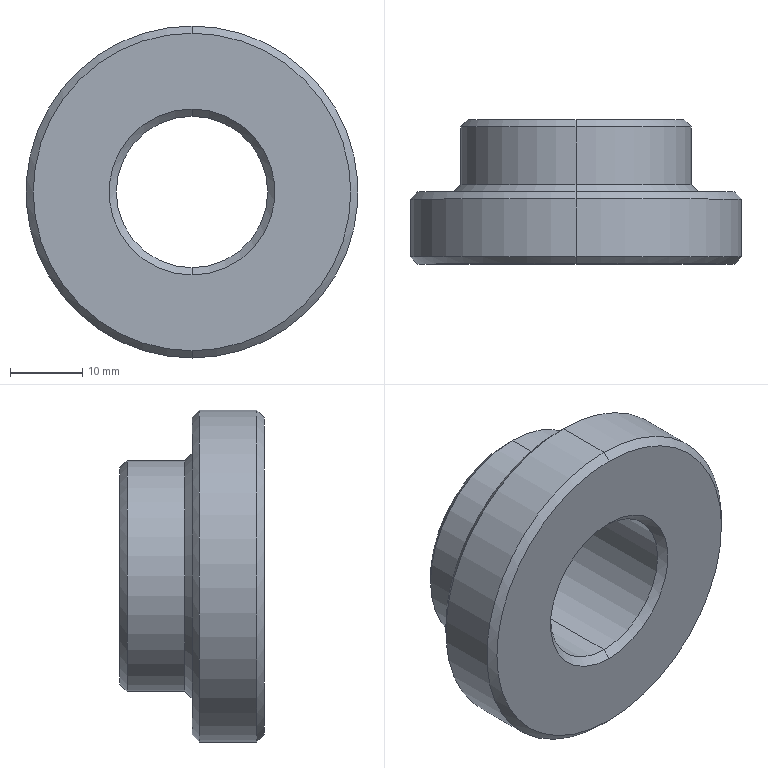Part | SolidWorks | features Chamfer 2, ICE 2, Extrusion 1 | 1 solid | 21 faces | box 46 x 20 x 46 mm | volume 17526 mm3 | cone 12 | cylinder 6 | plane 3 | commonest cylinder face diameters 21 x2 32 x2 46 x2
STEP:
#1=CARTESIAN_POINT('',(0.,1.,10.5));
#2=VERTEX_POINT('',#1);
#3=CARTESIAN_POINT('',(0.,1.,-10.5));
#4=VERTEX_POINT('',#3);
#5=CARTESIAN_POINT('',(0.,1.,0.));
#6=DIRECTION('',(0.,-1.,0.));
#7=DIRECTION('',(0.,0.,1.));
#8=AXIS2_PLACEMENT_3D('',#5,#6,#7);
#9=CIRCLE('',#8,10.5);
#10=EDGE_CURVE('',#2,#4,#9,.T.);
#11=ORIENTED_EDGE('',*,*,#10,.F.);
#12=CARTESIAN_POINT('',(0.,0.,11.5));
#13=VERTEX_POINT('',#12);
#14=CARTESIAN_POINT('',(0.,0.,11.5));
#15=DIRECTION('',(0.,-0.7071,0.7071));
#16=VECTOR('',#15,1000.);
#17=LINE('',#14,#16);
#18=EDGE_CURVE('',#2,#13,#17,.T.);
#19=ORIENTED_EDGE('',*,*,#18,.T.);
#20=CARTESIAN_POINT('',(0.,0.,-11.5));
#21=VERTEX_POINT('',#20);
#22=CARTESIAN_POINT('',(0.,0.,0.));
#23=DIRECTION('',(0.,1.,0.));
#24=DIRECTION('',(0.,0.,1.));
#25=AXIS2_PLACEMENT_3D('',#22,#23,#24);
#26=CIRCLE('',#25,11.5);
#27=EDGE_CURVE('',#21,#13,#26,.T.);
#28=ORIENTED_EDGE('',*,*,#27,.F.);
#29=CARTESIAN_POINT('',(0.,0.,-11.5));
#30=DIRECTION('',(0.,-0.7071,-0.7071));
#31=VECTOR('',#30,1000.);
#32=LINE('',#29,#31);
#33=EDGE_CURVE('',#4,#21,#32,.T.);
#34=ORIENTED_EDGE('',*,*,#33,.F.);
#35=EDGE_LOOP('',(#11,#19,#28,#34));
#36=FACE_OUTER_BOUND('',#35,.T.);
#37=CARTESIAN_POINT('',(0.,0.,0.));
#38=DIRECTION('',(0.,-1.,0.));
#39=DIRECTION('',(0.,0.,-1.));
#40=AXIS2_PLACEMENT_3D('',#37,#38,#39);
#41=CONICAL_SURFACE('',#40,11.5,0.7854);
#42=ADVANCED_FACE('',(#36),#41,.F.);
#43=CARTESIAN_POINT('',(0.,19.,-10.5));
#44=VERTEX_POINT('',#43);
#45=CARTESIAN_POINT('',(0.,19.,10.5));
#46=VERTEX_POINT('',#45);
#47=CARTESIAN_POINT('',(0.,19.,0.));
#48=DIRECTION('',(0.,1.,0.));
#49=DIRECTION('',(0.,0.,1.));
#50=AXIS2_PLACEMENT_3D('',#47,#48,#49);
#51=CIRCLE('',#50,10.5);
#52=EDGE_CURVE('',#44,#46,#51,.T.);
#53=ORIENTED_EDGE('',*,*,#52,.F.);
#54=CARTESIAN_POINT('',(0.,20.,-11.5));
#55=VERTEX_POINT('',#54);
#56=CARTESIAN_POINT('',(0.,19.,-10.5));
#57=DIRECTION('',(0.,0.7071,-0.7071));
#58=VECTOR('',#57,1000.);
#59=LINE('',#56,#58);
#60=EDGE_CURVE('',#44,#55,#59,.T.);
#61=ORIENTED_EDGE('',*,*,#60,.T.);
#62=CARTESIAN_POINT('',(0.,20.,11.5));
#63=VERTEX_POINT('',#62);
#64=CARTESIAN_POINT('',(0.,20.,0.));
#65=DIRECTION('',(0.,-1.,0.));
#66=DIRECTION('',(0.,0.,1.));
#67=AXIS2_PLACEMENT_3D('',#64,#65,#66);
#68=CIRCLE('',#67,11.5);
#69=EDGE_CURVE('',#63,#55,#68,.T.);
#70=ORIENTED_EDGE('',*,*,#69,.F.);
#71=CARTESIAN_POINT('',(0.,19.,10.5));
#72=DIRECTION('',(0.,0.7071,0.7071));
#73=VECTOR('',#72,1000.);
#74=LINE('',#71,#73);
#75=EDGE_CURVE('',#46,#63,#74,.T.);
#76=ORIENTED_EDGE('',*,*,#75,.F.);
#77=EDGE_LOOP('',(#53,#61,#70,#76));
#78=FACE_OUTER_BOUND('',#77,.T.);
#79=CARTESIAN_POINT('',(0.,19.,0.));
#80=DIRECTION('',(0.,1.,0.));
#81=DIRECTION('',(0.,0.,1.));
#82=AXIS2_PLACEMENT_3D('',#79,#80,#81);
#83=CONICAL_SURFACE('',#82,10.5,0.7854);
#84=ADVANCED_FACE('',(#78),#83,.F.);
#85=CARTESIAN_POINT('',(0.,20.,15.));
#86=VERTEX_POINT('',#85);
#87=CARTESIAN_POINT('',(0.,20.,-15.));
#88=VERTEX_POINT('',#87);
#89=CARTESIAN_POINT('',(0.,20.,0.));
#90=DIRECTION('',(0.,1.,0.));
#91=DIRECTION('',(0.,0.,1.));
#92=AXIS2_PLACEMENT_3D('',#89,#90,#91);
#93=CIRCLE('',#92,15.);
#94=EDGE_CURVE('',#86,#88,#93,.T.);
#95=ORIENTED_EDGE('',*,*,#94,.F.);
#96=CARTESIAN_POINT('',(0.,19.,16.));
#97=VERTEX_POINT('',#96);
#98=CARTESIAN_POINT('',(0.,20.,15.));
#99=DIRECTION('',(0.,-0.7071,0.7071));
#100=VECTOR('',#99,1000.);
#101=LINE('',#98,#100);
#102=EDGE_CURVE('',#86,#97,#101,.T.);
#103=ORIENTED_EDGE('',*,*,#102,.T.);
#104=CARTESIAN_POINT('',(0.,19.,-16.));
#105=VERTEX_POINT('',#104);
#106=CARTESIAN_POINT('',(0.,19.,0.));
#107=DIRECTION('',(0.,-1.,0.));
#108=DIRECTION('',(0.,0.,1.));
#109=AXIS2_PLACEMENT_3D('',#106,#107,#108);
#110=CIRCLE('',#109,16.);
#111=EDGE_CURVE('',#105,#97,#110,.T.);
#112=ORIENTED_EDGE('',*,*,#111,.F.);
#113=CARTESIAN_POINT('',(0.,20.,-15.));
#114=DIRECTION('',(0.,-0.7071,-0.7071));
#115=VECTOR('',#114,1000.);
#116=LINE('',#113,#115);
#117=EDGE_CURVE('',#88,#105,#116,.T.);
#118=ORIENTED_EDGE('',*,*,#117,.F.);
#119=EDGE_LOOP('',(#95,#103,#112,#118));
#120=FACE_OUTER_BOUND('',#119,.T.);
#121=CARTESIAN_POINT('',(0.,20.,0.));
#122=DIRECTION('',(0.,-1.,0.));
#123=DIRECTION('',(0.,0.,-1.));
#124=AXIS2_PLACEMENT_3D('',#121,#122,#123);
#125=CONICAL_SURFACE('',#124,15.,0.7854);
#126=ADVANCED_FACE('',(#120),#125,.T.);
#127=CARTESIAN_POINT('',(0.,11.,16.));
#128=VERTEX_POINT('',#127);
#129=CARTESIAN_POINT('',(0.,11.,-16.));
#130=VERTEX_POINT('',#129);
#131=CARTESIAN_POINT('',(0.,11.,0.));
#132=DIRECTION('',(0.,1.,0.));
#133=DIRECTION('',(0.,0.,1.));
#134=AXIS2_PLACEMENT_3D('',#131,#132,#133);
#135=CIRCLE('',#134,16.);
#136=EDGE_CURVE('',#128,#130,#135,.T.);
#137=ORIENTED_EDGE('',*,*,#136,.F.);
#138=CARTESIAN_POINT('',(0.,10.,17.));
#139=VERTEX_POINT('',#138);
#140=CARTESIAN_POINT('',(0.,11.,16.));
#141=DIRECTION('',(0.,-0.7071,0.7071));
#142=VECTOR('',#141,1000.);
#143=LINE('',#140,#142);
#144=EDGE_CURVE('',#128,#139,#143,.T.);
#145=ORIENTED_EDGE('',*,*,#144,.T.);
#146=CARTESIAN_POINT('',(0.,10.,-17.));
#147=VERTEX_POINT('',#146);
#148=CARTESIAN_POINT('',(0.,10.,0.));
#149=DIRECTION('',(0.,-1.,0.));
#150=DIRECTION('',(0.,0.,1.));
#151=AXIS2_PLACEMENT_3D('',#148,#149,#150);
#152=CIRCLE('',#151,17.);
#153=EDGE_CURVE('',#147,#139,#152,.T.);
#154=ORIENTED_EDGE('',*,*,#153,.F.);
#155=CARTESIAN_POINT('',(0.,11.,-16.));
#156=DIRECTION('',(0.,-0.7071,-0.7071));
#157=VECTOR('',#156,1000.);
#158=LINE('',#155,#157);
#159=EDGE_CURVE('',#130,#147,#158,.T.);
#160=ORIENTED_EDGE('',*,*,#159,.F.);
#161=EDGE_LOOP('',(#137,#145,#154,#160));
#162=FACE_OUTER_BOUND('',#161,.T.);
#163=CARTESIAN_POINT('',(0.,11.,0.));
#164=DIRECTION('',(0.,-1.,0.));
#165=DIRECTION('',(0.,0.,-1.));
#166=AXIS2_PLACEMENT_3D('',#163,#164,#165);
#167=CONICAL_SURFACE('',#166,16.,0.7854);
#168=ADVANCED_FACE('',(#162),#167,.T.);
#169=CARTESIAN_POINT('',(0.,10.,22.));
#170=VERTEX_POINT('',#169);
#171=CARTESIAN_POINT('',(0.,10.,-22.));
#172=VERTEX_POINT('',#171);
#173=CARTESIAN_POINT('',(0.,10.,0.));
#174=DIRECTION('',(0.,1.,0.));
#175=DIRECTION('',(0.,0.,1.));
#176=AXIS2_PLACEMENT_3D('',#173,#174,#175);
#177=CIRCLE('',#176,22.);
#178=EDGE_CURVE('',#170,#172,#177,.T.);
#179=ORIENTED_EDGE('',*,*,#178,.F.);
#180=CARTESIAN_POINT('',(0.,9.,23.));
#181=VERTEX_POINT('',#180);
#182=CARTESIAN_POINT('',(0.,10.,22.));
#183=DIRECTION('',(0.,-0.7071,0.7071));
#184=VECTOR('',#183,1000.);
#185=LINE('',#182,#184);
#186=EDGE_CURVE('',#170,#181,#185,.T.);
#187=ORIENTED_EDGE('',*,*,#186,.T.);
#188=CARTESIAN_POINT('',(0.,9.,-23.));
#189=VERTEX_POINT('',#188);
#190=CARTESIAN_POINT('',(0.,9.,0.));
#191=DIRECTION('',(0.,-1.,0.));
#192=DIRECTION('',(0.,0.,1.));
#193=AXIS2_PLACEMENT_3D('',#190,#191,#192);
#194=CIRCLE('',#193,23.);
#195=EDGE_CURVE('',#189,#181,#194,.T.);
#196=ORIENTED_EDGE('',*,*,#195,.F.);
#197=CARTESIAN_POINT('',(0.,10.,-22.));
#198=DIRECTION('',(0.,-0.7071,-0.7071));
#199=VECTOR('',#198,1000.);
#200=LINE('',#197,#199);
#201=EDGE_CURVE('',#172,#189,#200,.T.);
#202=ORIENTED_EDGE('',*,*,#201,.F.);
#203=EDGE_LOOP('',(#179,#187,#196,#202));
#204=FACE_OUTER_BOUND('',#203,.T.);
#205=CARTESIAN_POINT('',(0.,10.,0.));
#206=DIRECTION('',(0.,-1.,0.));
#207=DIRECTION('',(0.,0.,-1.));
#208=AXIS2_PLACEMENT_3D('',#205,#206,#207);
#209=CONICAL_SURFACE('',#208,22.,0.7854);
#210=ADVANCED_FACE('',(#204),#209,.T.);
#211=CARTESIAN_POINT('',(0.,0.,-22.));
#212=VERTEX_POINT('',#211);
#213=CARTESIAN_POINT('',(0.,0.,22.));
#214=VERTEX_POINT('',#213);
#215=CARTESIAN_POINT('',(0.,0.,0.));
#216=DIRECTION('',(0.,-1.,0.));
#217=DIRECTION('',(0.,0.,1.));
#218=AXIS2_PLACEMENT_3D('',#215,#216,#217);
#219=CIRCLE('',#218,22.);
#220=EDGE_CURVE('',#212,#214,#219,.T.);
#221=ORIENTED_EDGE('',*,*,#220,.F.);
#222=CARTESIAN_POINT('',(0.,1.,-23.));
#223=VERTEX_POINT('',#222);
#224=CARTESIAN_POINT('',(0.,1.,-23.));
#225=DIRECTION('',(0.,0.7071,-0.7071));
#226=VECTOR('',#225,1000.);
#227=LINE('',#224,#226);
#228=EDGE_CURVE('',#212,#223,#227,.T.);
#229=ORIENTED_EDGE('',*,*,#228,.T.);
#230=CARTESIAN_POINT('',(0.,1.,23.));
#231=VERTEX_POINT('',#230);
#232=CARTESIAN_POINT('',(0.,1.,0.));
#233=DIRECTION('',(0.,1.,0.));
#234=DIRECTION('',(0.,0.,1.));
#235=AXIS2_PLACEMENT_3D('',#232,#233,#234);
#236=CIRCLE('',#235,23.);
#237=EDGE_CURVE('',#231,#223,#236,.T.);
#238=ORIENTED_EDGE('',*,*,#237,.F.);
#239=CARTESIAN_POINT('',(0.,1.,23.));
#240=DIRECTION('',(0.,0.7071,0.7071));
#241=VECTOR('',#240,1000.);
#242=LINE('',#239,#241);
#243=EDGE_CURVE('',#214,#231,#242,.T.);
#244=ORIENTED_EDGE('',*,*,#243,.F.);
#245=EDGE_LOOP('',(#221,#229,#238,#244));
#246=FACE_OUTER_BOUND('',#245,.T.);
#247=CARTESIAN_POINT('',(0.,1.,0.));
#248=DIRECTION('',(0.,1.,0.));
#249=DIRECTION('',(0.,0.,1.));
#250=AXIS2_PLACEMENT_3D('',#247,#248,#249);
#251=CONICAL_SURFACE('',#250,23.,0.7854);
#252=ADVANCED_FACE('',(#246),#251,.T.);
#253=ORIENTED_EDGE('',*,*,#10,.T.);
#254=CARTESIAN_POINT('',(0.,0.,-10.5));
#255=DIRECTION('',(0.,1.,0.));
#256=VECTOR('',#255,1000.);
#257=LINE('',#254,#256);
#258=EDGE_CURVE('',#4,#44,#257,.T.);
#259=ORIENTED_EDGE('',*,*,#258,.T.);
#260=ORIENTED_EDGE('',*,*,#52,.T.);
#261=CARTESIAN_POINT('',(0.,0.,10.5));
#262=DIRECTION('',(0.,1.,0.));
#263=VECTOR('',#262,1000.);
#264=LINE('',#261,#263);
#265=EDGE_CURVE('',#2,#46,#264,.T.);
#266=ORIENTED_EDGE('',*,*,#265,.F.);
#267=EDGE_LOOP('',(#253,#259,#260,#266));
#268=FACE_OUTER_BOUND('',#267,.T.);
#269=CARTESIAN_POINT('',(0.,0.,0.));
#270=DIRECTION('',(0.,1.,0.));
#271=DIRECTION('',(0.,0.,1.));
#272=AXIS2_PLACEMENT_3D('',#269,#270,#271);
#273=CYLINDRICAL_SURFACE('',#272,10.5);
#274=ADVANCED_FACE('',(#268),#273,.F.);
#275=ORIENTED_EDGE('',*,*,#111,.T.);
#276=CARTESIAN_POINT('',(0.,20.,16.));
#277=DIRECTION('',(0.,-1.,0.));
#278=VECTOR('',#277,1000.);
#279=LINE('',#276,#278);
#280=EDGE_CURVE('',#97,#128,#279,.T.);
#281=ORIENTED_EDGE('',*,*,#280,.T.);
#282=ORIENTED_EDGE('',*,*,#136,.T.);
#283=CARTESIAN_POINT('',(0.,20.,-16.));
#284=DIRECTION('',(0.,-1.,0.));
#285=VECTOR('',#284,1000.);
#286=LINE('',#283,#285);
#287=EDGE_CURVE('',#105,#130,#286,.T.);
#288=ORIENTED_EDGE('',*,*,#287,.F.);
#289=EDGE_LOOP('',(#275,#281,#282,#288));
#290=FACE_OUTER_BOUND('',#289,.T.);
#291=CARTESIAN_POINT('',(0.,20.,0.));
#292=DIRECTION('',(0.,-1.,0.));
#293=DIRECTION('',(0.,0.,-1.));
#294=AXIS2_PLACEMENT_3D('',#291,#292,#293);
#295=CYLINDRICAL_SURFACE('',#294,16.);
#296=ADVANCED_FACE('',(#290),#295,.T.);
#297=ORIENTED_EDGE('',*,*,#195,.T.);
#298=CARTESIAN_POINT('',(0.,10.,23.));
#299=DIRECTION('',(0.,-1.,0.));
#300=VECTOR('',#299,1000.);
#301=LINE('',#298,#300);
#302=EDGE_CURVE('',#181,#231,#301,.T.);
#303=ORIENTED_EDGE('',*,*,#302,.T.);
#304=ORIENTED_EDGE('',*,*,#237,.T.);
#305=CARTESIAN_POINT('',(0.,10.,-23.));
#306=DIRECTION('',(0.,-1.,0.));
#307=VECTOR('',#306,1000.);
#308=LINE('',#305,#307);
#309=EDGE_CURVE('',#189,#223,#308,.T.);
#310=ORIENTED_EDGE('',*,*,#309,.F.);
#311=EDGE_LOOP('',(#297,#303,#304,#310));
#312=FACE_OUTER_BOUND('',#311,.T.);
#313=CARTESIAN_POINT('',(0.,10.,0.));
#314=DIRECTION('',(0.,-1.,0.));
#315=DIRECTION('',(0.,0.,-1.));
#316=AXIS2_PLACEMENT_3D('',#313,#314,#315);
#317=CYLINDRICAL_SURFACE('',#316,23.);
#318=ADVANCED_FACE('',(#312),#317,.T.);
#319=ORIENTED_EDGE('',*,*,#302,.F.);
#320=CARTESIAN_POINT('',(0.,9.,0.));
#321=DIRECTION('',(0.,-1.,0.));
#322=DIRECTION('',(0.,0.,1.));
#323=AXIS2_PLACEMENT_3D('',#320,#321,#322);
#324=CIRCLE('',#323,23.);
#325=EDGE_CURVE('',#181,#189,#324,.T.);
#326=ORIENTED_EDGE('',*,*,#325,.T.);
#327=ORIENTED_EDGE('',*,*,#309,.T.);
#328=CARTESIAN_POINT('',(0.,1.,0.));
#329=DIRECTION('',(0.,1.,0.));
#330=DIRECTION('',(0.,0.,1.));
#331=AXIS2_PLACEMENT_3D('',#328,#329,#330);
#332=CIRCLE('',#331,23.);
#333=EDGE_CURVE('',#223,#231,#332,.T.);
#334=ORIENTED_EDGE('',*,*,#333,.T.);
#335=EDGE_LOOP('',(#319,#326,#327,#334));
#336=FACE_OUTER_BOUND('',#335,.T.);
#337=CARTESIAN_POINT('',(0.,10.,0.));
#338=DIRECTION('',(0.,-1.,0.));
#339=DIRECTION('',(0.,0.,-1.));
#340=AXIS2_PLACEMENT_3D('',#337,#338,#339);
#341=CYLINDRICAL_SURFACE('',#340,23.);
#342=ADVANCED_FACE('',(#336),#341,.T.);
#343=CARTESIAN_POINT('',(0.,10.,0.));
#344=DIRECTION('',(0.,1.,0.));
#345=DIRECTION('',(0.,0.,1.));
#346=AXIS2_PLACEMENT_3D('',#343,#344,#345);
#347=CIRCLE('',#346,22.);
#348=EDGE_CURVE('',#172,#170,#347,.T.);
#349=ORIENTED_EDGE('',*,*,#348,.T.);
#350=ORIENTED_EDGE('',*,*,#178,.T.);
#351=EDGE_LOOP('',(#349,#350));
#352=FACE_OUTER_BOUND('',#351,.T.);
#353=ORIENTED_EDGE('',*,*,#153,.T.);
#354=CARTESIAN_POINT('',(0.,10.,0.));
#355=DIRECTION('',(0.,-1.,0.));
#356=DIRECTION('',(0.,0.,1.));
#357=AXIS2_PLACEMENT_3D('',#354,#355,#356);
#358=CIRCLE('',#357,17.);
#359=EDGE_CURVE('',#139,#147,#358,.T.);
#360=ORIENTED_EDGE('',*,*,#359,.T.);
#361=EDGE_LOOP('',(#353,#360));
#362=FACE_BOUND('',#361,.T.);
#363=CARTESIAN_POINT('',(0.,10.,0.));
#364=DIRECTION('',(0.,1.,0.));
#365=DIRECTION('',(0.,0.,1.));
#366=AXIS2_PLACEMENT_3D('',#363,#364,#365);
#367=PLANE('',#366);
#368=ADVANCED_FACE('',(#352,#362),#367,.T.);
#369=ORIENTED_EDGE('',*,*,#27,.T.);
#370=CARTESIAN_POINT('',(0.,0.,0.));
#371=DIRECTION('',(0.,1.,0.));
#372=DIRECTION('',(0.,0.,1.));
#373=AXIS2_PLACEMENT_3D('',#370,#371,#372);
#374=CIRCLE('',#373,11.5);
#375=EDGE_CURVE('',#13,#21,#374,.T.);
#376=ORIENTED_EDGE('',*,*,#375,.T.);
#377=EDGE_LOOP('',(#369,#376));
#378=FACE_BOUND('',#377,.T.);
#379=CARTESIAN_POINT('',(0.,0.,0.));
#380=DIRECTION('',(0.,-1.,0.));
#381=DIRECTION('',(0.,0.,1.));
#382=AXIS2_PLACEMENT_3D('',#379,#380,#381);
#383=CIRCLE('',#382,22.);
#384=EDGE_CURVE('',#214,#212,#383,.T.);
#385=ORIENTED_EDGE('',*,*,#384,.T.);
#386=ORIENTED_EDGE('',*,*,#220,.T.);
#387=EDGE_LOOP('',(#385,#386));
#388=FACE_OUTER_BOUND('',#387,.T.);
#389=CARTESIAN_POINT('',(0.,0.,0.));
#390=DIRECTION('',(0.,1.,0.));
#391=DIRECTION('',(0.,0.,1.));
#392=AXIS2_PLACEMENT_3D('',#389,#390,#391);
#393=PLANE('',#392);
#394=ADVANCED_FACE('',(#378,#388),#393,.F.);
#395=ORIENTED_EDGE('',*,*,#280,.F.);
#396=CARTESIAN_POINT('',(0.,19.,0.));
#397=DIRECTION('',(0.,-1.,0.));
#398=DIRECTION('',(0.,0.,1.));
#399=AXIS2_PLACEMENT_3D('',#396,#397,#398);
#400=CIRCLE('',#399,16.);
#401=EDGE_CURVE('',#97,#105,#400,.T.);
#402=ORIENTED_EDGE('',*,*,#401,.T.);
#403=ORIENTED_EDGE('',*,*,#287,.T.);
#404=CARTESIAN_POINT('',(0.,11.,0.));
#405=DIRECTION('',(0.,1.,0.));
#406=DIRECTION('',(0.,0.,1.));
#407=AXIS2_PLACEMENT_3D('',#404,#405,#406);
#408=CIRCLE('',#407,16.);
#409=EDGE_CURVE('',#130,#128,#408,.T.);
#410=ORIENTED_EDGE('',*,*,#409,.T.);
#411=EDGE_LOOP('',(#395,#402,#403,#410));
#412=FACE_OUTER_BOUND('',#411,.T.);
#413=CARTESIAN_POINT('',(0.,20.,0.));
#414=DIRECTION('',(0.,-1.,0.));
#415=DIRECTION('',(0.,0.,-1.));
#416=AXIS2_PLACEMENT_3D('',#413,#414,#415);
#417=CYLINDRICAL_SURFACE('',#416,16.);
#418=ADVANCED_FACE('',(#412),#417,.T.);
#419=CARTESIAN_POINT('',(0.,20.,0.));
#420=DIRECTION('',(0.,1.,0.));
#421=DIRECTION('',(0.,0.,1.));
#422=AXIS2_PLACEMENT_3D('',#419,#420,#421);
#423=CIRCLE('',#422,15.);
#424=EDGE_CURVE('',#88,#86,#423,.T.);
#425=ORIENTED_EDGE('',*,*,#424,.T.);
#426=ORIENTED_EDGE('',*,*,#94,.T.);
#427=EDGE_LOOP('',(#425,#426));
#428=FACE_OUTER_BOUND('',#427,.T.);
#429=ORIENTED_EDGE('',*,*,#69,.T.);
#430=CARTESIAN_POINT('',(0.,20.,0.));
#431=DIRECTION('',(0.,-1.,0.));
#432=DIRECTION('',(0.,0.,1.));
#433=AXIS2_PLACEMENT_3D('',#430,#431,#432);
#434=CIRCLE('',#433,11.5);
#435=EDGE_CURVE('',#55,#63,#434,.T.);
#436=ORIENTED_EDGE('',*,*,#435,.T.);
#437=EDGE_LOOP('',(#429,#436));
#438=FACE_BOUND('',#437,.T.);
#439=CARTESIAN_POINT('',(0.,20.,0.));
#440=DIRECTION('',(0.,1.,0.));
#441=DIRECTION('',(0.,0.,1.));
#442=AXIS2_PLACEMENT_3D('',#439,#440,#441);
#443=PLANE('',#442);
#444=ADVANCED_FACE('',(#428,#438),#443,.T.);
#445=ORIENTED_EDGE('',*,*,#258,.F.);
#446=CARTESIAN_POINT('',(0.,1.,0.));
#447=DIRECTION('',(0.,-1.,0.));
#448=DIRECTION('',(0.,0.,1.));
#449=AXIS2_PLACEMENT_3D('',#446,#447,#448);
#450=CIRCLE('',#449,10.5);
#451=EDGE_CURVE('',#4,#2,#450,.T.);
#452=ORIENTED_EDGE('',*,*,#451,.T.);
#453=ORIENTED_EDGE('',*,*,#265,.T.);
#454=CARTESIAN_POINT('',(0.,19.,0.));
#455=DIRECTION('',(0.,1.,0.));
#456=DIRECTION('',(0.,0.,1.));
#457=AXIS2_PLACEMENT_3D('',#454,#455,#456);
#458=CIRCLE('',#457,10.5);
#459=EDGE_CURVE('',#46,#44,#458,.T.);
#460=ORIENTED_EDGE('',*,*,#459,.T.);
#461=EDGE_LOOP('',(#445,#452,#453,#460));
#462=FACE_OUTER_BOUND('',#461,.T.);
#463=CARTESIAN_POINT('',(0.,0.,0.));
#464=DIRECTION('',(0.,1.,0.));
#465=DIRECTION('',(0.,0.,1.));
#466=AXIS2_PLACEMENT_3D('',#463,#464,#465);
#467=CYLINDRICAL_SURFACE('',#466,10.5);
#468=ADVANCED_FACE('',(#462),#467,.F.);
#469=ORIENTED_EDGE('',*,*,#228,.F.);
#470=ORIENTED_EDGE('',*,*,#384,.F.);
#471=ORIENTED_EDGE('',*,*,#243,.T.);
#472=ORIENTED_EDGE('',*,*,#333,.F.);
#473=EDGE_LOOP('',(#469,#470,#471,#472));
#474=FACE_OUTER_BOUND('',#473,.T.);
#475=CARTESIAN_POINT('',(0.,1.,0.));
#476=DIRECTION('',(0.,1.,0.));
#477=DIRECTION('',(0.,0.,1.));
#478=AXIS2_PLACEMENT_3D('',#475,#476,#477);
#479=CONICAL_SURFACE('',#478,23.,0.7854);
#480=ADVANCED_FACE('',(#474),#479,.T.);
#481=ORIENTED_EDGE('',*,*,#186,.F.);
#482=ORIENTED_EDGE('',*,*,#348,.F.);
#483=ORIENTED_EDGE('',*,*,#201,.T.);
#484=ORIENTED_EDGE('',*,*,#325,.F.);
#485=EDGE_LOOP('',(#481,#482,#483,#484));
#486=FACE_OUTER_BOUND('',#485,.T.);
#487=CARTESIAN_POINT('',(0.,10.,0.));
#488=DIRECTION('',(0.,-1.,0.));
#489=DIRECTION('',(0.,0.,-1.));
#490=AXIS2_PLACEMENT_3D('',#487,#488,#489);
#491=CONICAL_SURFACE('',#490,22.,0.7854);
#492=ADVANCED_FACE('',(#486),#491,.T.);
#493=ORIENTED_EDGE('',*,*,#144,.F.);
#494=ORIENTED_EDGE('',*,*,#409,.F.);
#495=ORIENTED_EDGE('',*,*,#159,.T.);
#496=ORIENTED_EDGE('',*,*,#359,.F.);
#497=EDGE_LOOP('',(#493,#494,#495,#496));
#498=FACE_OUTER_BOUND('',#497,.T.);
#499=CARTESIAN_POINT('',(0.,11.,0.));
#500=DIRECTION('',(0.,-1.,0.));
#501=DIRECTION('',(0.,0.,-1.));
#502=AXIS2_PLACEMENT_3D('',#499,#500,#501);
#503=CONICAL_SURFACE('',#502,16.,0.7854);
#504=ADVANCED_FACE('',(#498),#503,.T.);
#505=ORIENTED_EDGE('',*,*,#102,.F.);
#506=ORIENTED_EDGE('',*,*,#424,.F.);
#507=ORIENTED_EDGE('',*,*,#117,.T.);
#508=ORIENTED_EDGE('',*,*,#401,.F.);
#509=EDGE_LOOP('',(#505,#506,#507,#508));
#510=FACE_OUTER_BOUND('',#509,.T.);
#511=CARTESIAN_POINT('',(0.,20.,0.));
#512=DIRECTION('',(0.,-1.,0.));
#513=DIRECTION('',(0.,0.,-1.));
#514=AXIS2_PLACEMENT_3D('',#511,#512,#513);
#515=CONICAL_SURFACE('',#514,15.,0.7854);
#516=ADVANCED_FACE('',(#510),#515,.T.);
#517=ORIENTED_EDGE('',*,*,#60,.F.);
#518=ORIENTED_EDGE('',*,*,#459,.F.);
#519=ORIENTED_EDGE('',*,*,#75,.T.);
#520=ORIENTED_EDGE('',*,*,#435,.F.);
#521=EDGE_LOOP('',(#517,#518,#519,#520));
#522=FACE_OUTER_BOUND('',#521,.T.);
#523=CARTESIAN_POINT('',(0.,19.,0.));
#524=DIRECTION('',(0.,1.,0.));
#525=DIRECTION('',(0.,0.,1.));
#526=AXIS2_PLACEMENT_3D('',#523,#524,#525);
#527=CONICAL_SURFACE('',#526,10.5,0.7854);
#528=ADVANCED_FACE('',(#522),#527,.F.);
#529=ORIENTED_EDGE('',*,*,#18,.F.);
#530=ORIENTED_EDGE('',*,*,#451,.F.);
#531=ORIENTED_EDGE('',*,*,#33,.T.);
#532=ORIENTED_EDGE('',*,*,#375,.F.);
#533=EDGE_LOOP('',(#529,#530,#531,#532));
#534=FACE_OUTER_BOUND('',#533,.T.);
#535=CARTESIAN_POINT('',(0.,0.,0.));
#536=DIRECTION('',(0.,-1.,0.));
#537=DIRECTION('',(0.,0.,-1.));
#538=AXIS2_PLACEMENT_3D('',#535,#536,#537);
#539=CONICAL_SURFACE('',#538,11.5,0.7854);
#540=ADVANCED_FACE('',(#534),#539,.F.);
#541=CLOSED_SHELL('',(#42,#84,#126,#168,#210,#252,#274,#296,#318,#342,#368,#394,#418,#444,#468,#480,#492,#504,#516,#528,#540));
#542=MANIFOLD_SOLID_BREP('',#541);
#543=CARTESIAN_POINT('',(0.,0.,0.));
#544=DIRECTION('',(0.,0.,1.));
#545=DIRECTION('',(1.,0.,0.));
#546=AXIS2_PLACEMENT_3D('',#543,#544,#545);
#547=(LENGTH_UNIT()NAMED_UNIT(*)SI_UNIT(.MILLI.,.METRE.));
#548=UNCERTAINTY_MEASURE_WITH_UNIT(LENGTH_MEASURE(0.00001),#547,'','');
#549=(NAMED_UNIT(*)PLANE_ANGLE_UNIT()SI_UNIT($,.RADIAN.));
#550=(NAMED_UNIT(*)SI_UNIT($,.STERADIAN.)SOLID_ANGLE_UNIT());
#551=(GEOMETRIC_REPRESENTATION_CONTEXT(3)GLOBAL_UNCERTAINTY_ASSIGNED_CONTEXT((#548))GLOBAL_UNIT_ASSIGNED_CONTEXT((#547,#549,#550))REPRESENTATION_CONTEXT('',''));
#552=ADVANCED_BREP_SHAPE_REPRESENTATION('',(#542,#546),#551);